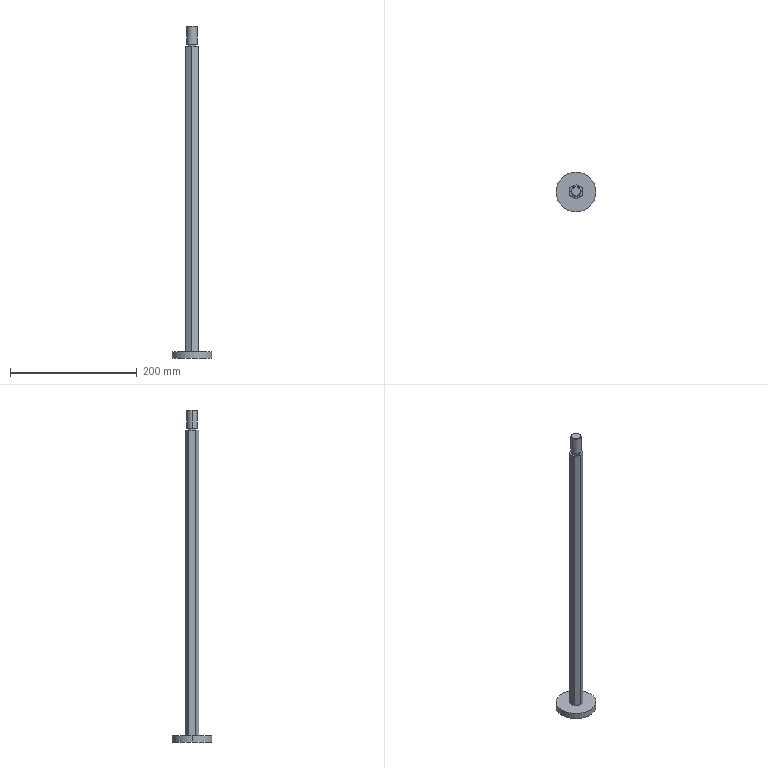Part | SolidWorks | features BaseBody 1 | 1 solid | 21 faces | box 63 x 63 x 524 mm | volume 188150 mm3 | plane 11 | cylinder 6 | cone 4 | commonest cylinder face diameters 14 x2 16 x2 63 x2
STEP:
#1=CARTESIAN_POINT('',(-242.,0.,321.531));
#2=VERTEX_POINT('',#1);
#3=CARTESIAN_POINT('',(-228.,0.,321.531));
#4=VERTEX_POINT('',#3);
#5=CARTESIAN_POINT('',(-235.,0.,321.531));
#6=DIRECTION('',(0.,0.,-1.));
#7=DIRECTION('',(-1.,0.,0.));
#8=AXIS2_PLACEMENT_3D('',#5,#6,#7);
#9=CIRCLE('',#8,7.);
#10=EDGE_CURVE('',#2,#4,#9,.T.);
#11=ORIENTED_EDGE('',*,*,#10,.T.);
#12=CARTESIAN_POINT('',(-228.,0.,319.281));
#13=VERTEX_POINT('',#12);
#14=CARTESIAN_POINT('',(-228.,0.,320.406));
#15=DIRECTION('',(0.,0.,-1.));
#16=VECTOR('',#15,1000.);
#17=LINE('',#14,#16);
#18=EDGE_CURVE('',#4,#13,#17,.T.);
#19=ORIENTED_EDGE('',*,*,#18,.T.);
#20=CARTESIAN_POINT('',(-242.,0.,319.281));
#21=VERTEX_POINT('',#20);
#22=CARTESIAN_POINT('',(-235.,0.,319.281));
#23=DIRECTION('',(0.,0.,-1.));
#24=DIRECTION('',(-1.,0.,0.));
#25=AXIS2_PLACEMENT_3D('',#22,#23,#24);
#26=CIRCLE('',#25,7.);
#27=EDGE_CURVE('',#21,#13,#26,.T.);
#28=ORIENTED_EDGE('',*,*,#27,.F.);
#29=CARTESIAN_POINT('',(-242.,0.,320.406));
#30=DIRECTION('',(0.,0.,-1.));
#31=VECTOR('',#30,1000.);
#32=LINE('',#29,#31);
#33=EDGE_CURVE('',#2,#21,#32,.T.);
#34=ORIENTED_EDGE('',*,*,#33,.F.);
#35=EDGE_LOOP('',(#11,#19,#28,#34));
#36=FACE_OUTER_BOUND('',#35,.T.);
#37=CARTESIAN_POINT('',(-235.,0.,320.406));
#38=DIRECTION('',(0.,0.,-1.));
#39=DIRECTION('',(-1.,0.,0.));
#40=AXIS2_PLACEMENT_3D('',#37,#38,#39);
#41=CYLINDRICAL_SURFACE('',#40,7.);
#42=ADVANCED_FACE('',(#36),#41,.T.);
#43=CARTESIAN_POINT('',(-203.5,0.,-162.719));
#44=VERTEX_POINT('',#43);
#45=CARTESIAN_POINT('',(-266.5,0.,-162.719));
#46=VERTEX_POINT('',#45);
#47=CARTESIAN_POINT('',(-235.,0.,-162.719));
#48=DIRECTION('',(0.,0.,1.));
#49=DIRECTION('',(-1.,0.,0.));
#50=AXIS2_PLACEMENT_3D('',#47,#48,#49);
#51=CIRCLE('',#50,31.5);
#52=EDGE_CURVE('',#44,#46,#51,.T.);
#53=ORIENTED_EDGE('',*,*,#52,.F.);
#54=CARTESIAN_POINT('',(-203.5,0.,-172.719));
#55=VERTEX_POINT('',#54);
#56=CARTESIAN_POINT('',(-203.5,0.,-167.719));
#57=DIRECTION('',(0.,0.,-1.));
#58=VECTOR('',#57,1000.);
#59=LINE('',#56,#58);
#60=EDGE_CURVE('',#44,#55,#59,.T.);
#61=ORIENTED_EDGE('',*,*,#60,.T.);
#62=CARTESIAN_POINT('',(-266.5,0.,-172.719));
#63=VERTEX_POINT('',#62);
#64=CARTESIAN_POINT('',(-235.,0.,-172.719));
#65=DIRECTION('',(0.,0.,1.));
#66=DIRECTION('',(-1.,0.,0.));
#67=AXIS2_PLACEMENT_3D('',#64,#65,#66);
#68=CIRCLE('',#67,31.5);
#69=EDGE_CURVE('',#55,#63,#68,.T.);
#70=ORIENTED_EDGE('',*,*,#69,.T.);
#71=CARTESIAN_POINT('',(-266.5,0.,-167.719));
#72=DIRECTION('',(0.,0.,-1.));
#73=VECTOR('',#72,1000.);
#74=LINE('',#71,#73);
#75=EDGE_CURVE('',#46,#63,#74,.T.);
#76=ORIENTED_EDGE('',*,*,#75,.F.);
#77=EDGE_LOOP('',(#53,#61,#70,#76));
#78=FACE_OUTER_BOUND('',#77,.T.);
#79=CARTESIAN_POINT('',(-235.,0.,-167.719));
#80=DIRECTION('',(0.,0.,-1.));
#81=DIRECTION('',(-1.,0.,0.));
#82=AXIS2_PLACEMENT_3D('',#79,#80,#81);
#83=CYLINDRICAL_SURFACE('',#82,31.5);
#84=ADVANCED_FACE('',(#78),#83,.T.);
#85=CARTESIAN_POINT('',(-242.08,0.,321.531));
#86=VERTEX_POINT('',#85);
#87=CARTESIAN_POINT('',(-227.92,0.,321.531));
#88=VERTEX_POINT('',#87);
#89=CARTESIAN_POINT('',(-235.,0.,321.531));
#90=DIRECTION('',(0.,0.,-1.));
#91=DIRECTION('',(1.,0.,0.));
#92=AXIS2_PLACEMENT_3D('',#89,#90,#91);
#93=CIRCLE('',#92,7.08);
#94=EDGE_CURVE('',#86,#88,#93,.T.);
#95=ORIENTED_EDGE('',*,*,#94,.F.);
#96=CARTESIAN_POINT('',(-243.,0.,322.451));
#97=VERTEX_POINT('',#96);
#98=CARTESIAN_POINT('',(-243.,0.,322.451));
#99=DIRECTION('',(-0.7071,0.,0.7071));
#100=VECTOR('',#99,1000.);
#101=LINE('',#98,#100);
#102=EDGE_CURVE('',#86,#97,#101,.T.);
#103=ORIENTED_EDGE('',*,*,#102,.T.);
#104=CARTESIAN_POINT('',(-227.,0.,322.451));
#105=VERTEX_POINT('',#104);
#106=CARTESIAN_POINT('',(-235.,0.,322.451));
#107=DIRECTION('',(0.,0.,-1.));
#108=DIRECTION('',(-0.866,-0.5,0.));
#109=AXIS2_PLACEMENT_3D('',#106,#107,#108);
#110=CIRCLE('',#109,8.);
#111=EDGE_CURVE('',#97,#105,#110,.T.);
#112=ORIENTED_EDGE('',*,*,#111,.T.);
#113=CARTESIAN_POINT('',(-227.,0.,322.451));
#114=DIRECTION('',(0.7071,0.,0.7071));
#115=VECTOR('',#114,1000.);
#116=LINE('',#113,#115);
#117=EDGE_CURVE('',#88,#105,#116,.T.);
#118=ORIENTED_EDGE('',*,*,#117,.F.);
#119=EDGE_LOOP('',(#95,#103,#112,#118));
#120=FACE_OUTER_BOUND('',#119,.T.);
#121=CARTESIAN_POINT('',(-235.,0.,322.451));
#122=DIRECTION('',(0.,0.,1.));
#123=DIRECTION('',(1.,0.,0.));
#124=AXIS2_PLACEMENT_3D('',#121,#122,#123);
#125=CONICAL_SURFACE('',#124,8.,0.7854);
#126=ADVANCED_FACE('',(#120),#125,.T.);
#127=CARTESIAN_POINT('',(-235.,8.,350.361));
#128=VERTEX_POINT('',#127);
#129=CARTESIAN_POINT('',(-227.,0.,350.361));
#130=VERTEX_POINT('',#129);
#131=CARTESIAN_POINT('',(-235.,0.,350.361));
#132=DIRECTION('',(0.,0.,-1.));
#133=DIRECTION('',(-1.,0.,0.));
#134=AXIS2_PLACEMENT_3D('',#131,#132,#133);
#135=CIRCLE('',#134,8.);
#136=EDGE_CURVE('',#128,#130,#135,.T.);
#137=ORIENTED_EDGE('',*,*,#136,.T.);
#138=CARTESIAN_POINT('',(-227.,0.,336.406));
#139=DIRECTION('',(0.,0.,-1.));
#140=VECTOR('',#139,1000.);
#141=LINE('',#138,#140);
#142=EDGE_CURVE('',#130,#105,#141,.T.);
#143=ORIENTED_EDGE('',*,*,#142,.T.);
#144=ORIENTED_EDGE('',*,*,#111,.F.);
#145=CARTESIAN_POINT('',(-243.,0.,350.361));
#146=VERTEX_POINT('',#145);
#147=CARTESIAN_POINT('',(-243.,0.,336.406));
#148=DIRECTION('',(0.,0.,-1.));
#149=VECTOR('',#148,1000.);
#150=LINE('',#147,#149);
#151=EDGE_CURVE('',#146,#97,#150,.T.);
#152=ORIENTED_EDGE('',*,*,#151,.F.);
#153=CARTESIAN_POINT('',(-235.,0.,350.361));
#154=DIRECTION('',(0.,0.,-1.));
#155=DIRECTION('',(-1.,0.,0.));
#156=AXIS2_PLACEMENT_3D('',#153,#154,#155);
#157=CIRCLE('',#156,8.);
#158=EDGE_CURVE('',#146,#128,#157,.T.);
#159=ORIENTED_EDGE('',*,*,#158,.T.);
#160=EDGE_LOOP('',(#137,#143,#144,#152,#159));
#161=FACE_OUTER_BOUND('',#160,.T.);
#162=CARTESIAN_POINT('',(-235.,0.,336.406));
#163=DIRECTION('',(0.,0.,-1.));
#164=DIRECTION('',(-1.,0.,0.));
#165=AXIS2_PLACEMENT_3D('',#162,#163,#164);
#166=CYLINDRICAL_SURFACE('',#165,8.);
#167=ADVANCED_FACE('',(#161),#166,.T.);
#168=CARTESIAN_POINT('',(-235.,7.08,351.281));
#169=VERTEX_POINT('',#168);
#170=CARTESIAN_POINT('',(-235.,-7.08,351.281));
#171=VERTEX_POINT('',#170);
#172=CARTESIAN_POINT('',(-235.,0.,351.281));
#173=DIRECTION('',(0.,0.,-1.));
#174=DIRECTION('',(0.,1.,0.));
#175=AXIS2_PLACEMENT_3D('',#172,#173,#174);
#176=CIRCLE('',#175,7.08);
#177=EDGE_CURVE('',#169,#171,#176,.T.);
#178=ORIENTED_EDGE('',*,*,#177,.T.);
#179=CARTESIAN_POINT('',(-235.,-8.,350.361));
#180=VERTEX_POINT('',#179);
#181=CARTESIAN_POINT('',(-235.,-8.,350.361));
#182=DIRECTION('',(0.,-0.7071,-0.7071));
#183=VECTOR('',#182,1000.);
#184=LINE('',#181,#183);
#185=EDGE_CURVE('',#171,#180,#184,.T.);
#186=ORIENTED_EDGE('',*,*,#185,.T.);
#187=CARTESIAN_POINT('',(-235.,0.,350.361));
#188=DIRECTION('',(0.,0.,-1.));
#189=DIRECTION('',(-1.,0.,0.));
#190=AXIS2_PLACEMENT_3D('',#187,#188,#189);
#191=CIRCLE('',#190,8.);
#192=EDGE_CURVE('',#130,#180,#191,.T.);
#193=ORIENTED_EDGE('',*,*,#192,.F.);
#194=ORIENTED_EDGE('',*,*,#136,.F.);
#195=CARTESIAN_POINT('',(-235.,8.,350.361));
#196=DIRECTION('',(0.,0.7071,-0.7071));
#197=VECTOR('',#196,1000.);
#198=LINE('',#195,#197);
#199=EDGE_CURVE('',#169,#128,#198,.T.);
#200=ORIENTED_EDGE('',*,*,#199,.F.);
#201=EDGE_LOOP('',(#178,#186,#193,#194,#200));
#202=FACE_OUTER_BOUND('',#201,.T.);
#203=CARTESIAN_POINT('',(-235.,0.,350.361));
#204=DIRECTION('',(0.,0.,-1.));
#205=DIRECTION('',(0.,1.,0.));
#206=AXIS2_PLACEMENT_3D('',#203,#204,#205);
#207=CONICAL_SURFACE('',#206,8.,0.7854);
#208=ADVANCED_FACE('',(#202),#207,.T.);
#209=CARTESIAN_POINT('',(-235.,-10.97,319.281));
#210=VERTEX_POINT('',#209);
#211=CARTESIAN_POINT('',(-225.5,-5.485,319.281));
#212=VERTEX_POINT('',#211);
#213=CARTESIAN_POINT('',(-225.5,-5.485,319.281));
#214=DIRECTION('',(0.866,0.5,0.));
#215=VECTOR('',#214,1000.);
#216=LINE('',#213,#215);
#217=EDGE_CURVE('',#210,#212,#216,.T.);
#218=ORIENTED_EDGE('',*,*,#217,.F.);
#219=CARTESIAN_POINT('',(-235.,-10.97,-162.719));
#220=VERTEX_POINT('',#219);
#221=CARTESIAN_POINT('',(-235.,-10.97,319.281));
#222=DIRECTION('',(0.,0.,1.));
#223=VECTOR('',#222,1000.);
#224=LINE('',#221,#223);
#225=EDGE_CURVE('',#220,#210,#224,.T.);
#226=ORIENTED_EDGE('',*,*,#225,.F.);
#227=CARTESIAN_POINT('',(-225.5,-5.485,-162.719));
#228=VERTEX_POINT('',#227);
#229=CARTESIAN_POINT('',(-225.5,-5.485,-162.719));
#230=DIRECTION('',(-0.866,-0.5,0.));
#231=VECTOR('',#230,1000.);
#232=LINE('',#229,#231);
#233=EDGE_CURVE('',#228,#220,#232,.T.);
#234=ORIENTED_EDGE('',*,*,#233,.F.);
#235=CARTESIAN_POINT('',(-225.5,-5.485,319.281));
#236=DIRECTION('',(0.,0.,-1.));
#237=VECTOR('',#236,1000.);
#238=LINE('',#235,#237);
#239=EDGE_CURVE('',#212,#228,#238,.T.);
#240=ORIENTED_EDGE('',*,*,#239,.F.);
#241=EDGE_LOOP('',(#218,#226,#234,#240));
#242=FACE_OUTER_BOUND('',#241,.T.);
#243=CARTESIAN_POINT('',(-225.5,-5.485,319.281));
#244=DIRECTION('',(-0.5,0.866,0.));
#245=DIRECTION('',(-0.866,-0.5,0.));
#246=AXIS2_PLACEMENT_3D('',#243,#244,#245);
#247=PLANE('',#246);
#248=ADVANCED_FACE('',(#242),#247,.F.);
#249=CARTESIAN_POINT('',(-225.5,5.485,319.281));
#250=VERTEX_POINT('',#249);
#251=CARTESIAN_POINT('',(-225.5,5.485,319.281));
#252=DIRECTION('',(0.,1.,0.));
#253=VECTOR('',#252,1000.);
#254=LINE('',#251,#253);
#255=EDGE_CURVE('',#212,#250,#254,.T.);
#256=ORIENTED_EDGE('',*,*,#255,.F.);
#257=ORIENTED_EDGE('',*,*,#239,.T.);
#258=CARTESIAN_POINT('',(-225.5,5.485,-162.719));
#259=VERTEX_POINT('',#258);
#260=CARTESIAN_POINT('',(-225.5,5.485,-162.719));
#261=DIRECTION('',(0.,-1.,0.));
#262=VECTOR('',#261,1000.);
#263=LINE('',#260,#262);
#264=EDGE_CURVE('',#259,#228,#263,.T.);
#265=ORIENTED_EDGE('',*,*,#264,.F.);
#266=CARTESIAN_POINT('',(-225.5,5.485,319.281));
#267=DIRECTION('',(0.,0.,-1.));
#268=VECTOR('',#267,1000.);
#269=LINE('',#266,#268);
#270=EDGE_CURVE('',#250,#259,#269,.T.);
#271=ORIENTED_EDGE('',*,*,#270,.F.);
#272=EDGE_LOOP('',(#256,#257,#265,#271));
#273=FACE_OUTER_BOUND('',#272,.T.);
#274=CARTESIAN_POINT('',(-225.5,5.485,319.281));
#275=DIRECTION('',(-1.,0.,0.));
#276=DIRECTION('',(0.,0.,1.));
#277=AXIS2_PLACEMENT_3D('',#274,#275,#276);
#278=PLANE('',#277);
#279=ADVANCED_FACE('',(#273),#278,.F.);
#280=CARTESIAN_POINT('',(-235.,10.97,319.281));
#281=VERTEX_POINT('',#280);
#282=CARTESIAN_POINT('',(-244.5,5.485,319.281));
#283=VERTEX_POINT('',#282);
#284=CARTESIAN_POINT('',(-235.,10.97,319.281));
#285=DIRECTION('',(-0.866,-0.5,0.));
#286=VECTOR('',#285,1000.);
#287=LINE('',#284,#286);
#288=EDGE_CURVE('',#281,#283,#287,.T.);
#289=ORIENTED_EDGE('',*,*,#288,.T.);
#290=CARTESIAN_POINT('',(-244.5,-5.485,319.281));
#291=VERTEX_POINT('',#290);
#292=CARTESIAN_POINT('',(-244.5,9.613,319.281));
#293=DIRECTION('',(0.,-1.,0.));
#294=VECTOR('',#293,1000.);
#295=LINE('',#292,#294);
#296=EDGE_CURVE('',#283,#291,#295,.T.);
#297=ORIENTED_EDGE('',*,*,#296,.T.);
#298=CARTESIAN_POINT('',(-244.5,-5.485,319.281));
#299=DIRECTION('',(0.866,-0.5,0.));
#300=VECTOR('',#299,1000.);
#301=LINE('',#298,#300);
#302=EDGE_CURVE('',#291,#210,#301,.T.);
#303=ORIENTED_EDGE('',*,*,#302,.T.);
#304=ORIENTED_EDGE('',*,*,#217,.T.);
#305=ORIENTED_EDGE('',*,*,#255,.T.);
#306=CARTESIAN_POINT('',(-225.5,5.485,319.281));
#307=DIRECTION('',(-0.866,0.5,0.));
#308=VECTOR('',#307,1000.);
#309=LINE('',#306,#308);
#310=EDGE_CURVE('',#250,#281,#309,.T.);
#311=ORIENTED_EDGE('',*,*,#310,.T.);
#312=EDGE_LOOP('',(#289,#297,#303,#304,#305,#311));
#313=FACE_OUTER_BOUND('',#312,.T.);
#314=ORIENTED_EDGE('',*,*,#27,.T.);
#315=CARTESIAN_POINT('',(-235.,0.,319.281));
#316=DIRECTION('',(0.,0.,-1.));
#317=DIRECTION('',(-1.,0.,0.));
#318=AXIS2_PLACEMENT_3D('',#315,#316,#317);
#319=CIRCLE('',#318,7.);
#320=EDGE_CURVE('',#13,#21,#319,.T.);
#321=ORIENTED_EDGE('',*,*,#320,.T.);
#322=EDGE_LOOP('',(#314,#321));
#323=FACE_BOUND('',#322,.T.);
#324=CARTESIAN_POINT('',(-240.55,9.613,319.281));
#325=DIRECTION('',(0.,0.,1.));
#326=DIRECTION('',(1.,0.,0.));
#327=AXIS2_PLACEMENT_3D('',#324,#325,#326);
#328=PLANE('',#327);
#329=ADVANCED_FACE('',(#313,#323),#328,.T.);
#330=ORIENTED_EDGE('',*,*,#302,.F.);
#331=CARTESIAN_POINT('',(-244.5,-5.485,-162.719));
#332=VERTEX_POINT('',#331);
#333=CARTESIAN_POINT('',(-244.5,-5.485,319.281));
#334=DIRECTION('',(0.,0.,1.));
#335=VECTOR('',#334,1000.);
#336=LINE('',#333,#335);
#337=EDGE_CURVE('',#332,#291,#336,.T.);
#338=ORIENTED_EDGE('',*,*,#337,.F.);
#339=CARTESIAN_POINT('',(-235.,-10.97,-162.719));
#340=DIRECTION('',(-0.866,0.5,0.));
#341=VECTOR('',#340,1000.);
#342=LINE('',#339,#341);
#343=EDGE_CURVE('',#220,#332,#342,.T.);
#344=ORIENTED_EDGE('',*,*,#343,.F.);
#345=ORIENTED_EDGE('',*,*,#225,.T.);
#346=EDGE_LOOP('',(#330,#338,#344,#345));
#347=FACE_OUTER_BOUND('',#346,.T.);
#348=CARTESIAN_POINT('',(-235.,-10.97,319.281));
#349=DIRECTION('',(0.5,0.866,0.));
#350=DIRECTION('',(-0.866,0.5,0.));
#351=AXIS2_PLACEMENT_3D('',#348,#349,#350);
#352=PLANE('',#351);
#353=ADVANCED_FACE('',(#347),#352,.F.);
#354=ORIENTED_EDGE('',*,*,#343,.T.);
#355=CARTESIAN_POINT('',(-244.5,5.485,-162.719));
#356=VERTEX_POINT('',#355);
#357=CARTESIAN_POINT('',(-244.5,20.222,-162.719));
#358=DIRECTION('',(0.,1.,0.));
#359=VECTOR('',#358,1000.);
#360=LINE('',#357,#359);
#361=EDGE_CURVE('',#332,#356,#360,.T.);
#362=ORIENTED_EDGE('',*,*,#361,.T.);
#363=CARTESIAN_POINT('',(-235.,10.97,-162.719));
#364=VERTEX_POINT('',#363);
#365=CARTESIAN_POINT('',(-244.5,5.485,-162.719));
#366=DIRECTION('',(0.866,0.5,0.));
#367=VECTOR('',#366,1000.);
#368=LINE('',#365,#367);
#369=EDGE_CURVE('',#356,#364,#368,.T.);
#370=ORIENTED_EDGE('',*,*,#369,.T.);
#371=CARTESIAN_POINT('',(-235.,10.97,-162.719));
#372=DIRECTION('',(0.866,-0.5,0.));
#373=VECTOR('',#372,1000.);
#374=LINE('',#371,#373);
#375=EDGE_CURVE('',#364,#259,#374,.T.);
#376=ORIENTED_EDGE('',*,*,#375,.T.);
#377=ORIENTED_EDGE('',*,*,#264,.T.);
#378=ORIENTED_EDGE('',*,*,#233,.T.);
#379=EDGE_LOOP('',(#354,#362,#370,#376,#377,#378));
#380=FACE_BOUND('',#379,.T.);
#381=CARTESIAN_POINT('',(-235.,0.,-162.719));
#382=DIRECTION('',(0.,0.,1.));
#383=DIRECTION('',(-1.,0.,0.));
#384=AXIS2_PLACEMENT_3D('',#381,#382,#383);
#385=CIRCLE('',#384,31.5);
#386=EDGE_CURVE('',#46,#44,#385,.T.);
#387=ORIENTED_EDGE('',*,*,#386,.T.);
#388=ORIENTED_EDGE('',*,*,#52,.T.);
#389=EDGE_LOOP('',(#387,#388));
#390=FACE_OUTER_BOUND('',#389,.T.);
#391=CARTESIAN_POINT('',(-246.675,20.222,-162.719));
#392=DIRECTION('',(0.,0.,1.));
#393=DIRECTION('',(1.,0.,0.));
#394=AXIS2_PLACEMENT_3D('',#391,#392,#393);
#395=PLANE('',#394);
#396=ADVANCED_FACE('',(#380,#390),#395,.T.);
#397=ORIENTED_EDGE('',*,*,#310,.F.);
#398=ORIENTED_EDGE('',*,*,#270,.T.);
#399=ORIENTED_EDGE('',*,*,#375,.F.);
#400=CARTESIAN_POINT('',(-235.,10.97,319.281));
#401=DIRECTION('',(0.,0.,-1.));
#402=VECTOR('',#401,1000.);
#403=LINE('',#400,#402);
#404=EDGE_CURVE('',#281,#364,#403,.T.);
#405=ORIENTED_EDGE('',*,*,#404,.F.);
#406=EDGE_LOOP('',(#397,#398,#399,#405));
#407=FACE_OUTER_BOUND('',#406,.T.);
#408=CARTESIAN_POINT('',(-235.,10.97,319.281));
#409=DIRECTION('',(-0.5,-0.866,0.));
#410=DIRECTION('',(0.866,-0.5,0.));
#411=AXIS2_PLACEMENT_3D('',#408,#409,#410);
#412=PLANE('',#411);
#413=ADVANCED_FACE('',(#407),#412,.F.);
#414=ORIENTED_EDGE('',*,*,#296,.F.);
#415=CARTESIAN_POINT('',(-244.5,5.485,319.281));
#416=DIRECTION('',(0.,0.,1.));
#417=VECTOR('',#416,1000.);
#418=LINE('',#415,#417);
#419=EDGE_CURVE('',#356,#283,#418,.T.);
#420=ORIENTED_EDGE('',*,*,#419,.F.);
#421=ORIENTED_EDGE('',*,*,#361,.F.);
#422=ORIENTED_EDGE('',*,*,#337,.T.);
#423=EDGE_LOOP('',(#414,#420,#421,#422));
#424=FACE_OUTER_BOUND('',#423,.T.);
#425=CARTESIAN_POINT('',(-244.5,-5.485,319.281));
#426=DIRECTION('',(1.,0.,0.));
#427=DIRECTION('',(0.,0.,-1.));
#428=AXIS2_PLACEMENT_3D('',#425,#426,#427);
#429=PLANE('',#428);
#430=ADVANCED_FACE('',(#424),#429,.F.);
#431=ORIENTED_EDGE('',*,*,#288,.F.);
#432=ORIENTED_EDGE('',*,*,#404,.T.);
#433=ORIENTED_EDGE('',*,*,#369,.F.);
#434=ORIENTED_EDGE('',*,*,#419,.T.);
#435=EDGE_LOOP('',(#431,#432,#433,#434));
#436=FACE_OUTER_BOUND('',#435,.T.);
#437=CARTESIAN_POINT('',(-244.5,5.485,319.281));
#438=DIRECTION('',(0.5,-0.866,0.));
#439=DIRECTION('',(0.866,0.5,0.));
#440=AXIS2_PLACEMENT_3D('',#437,#438,#439);
#441=PLANE('',#440);
#442=ADVANCED_FACE('',(#436),#441,.F.);
#443=ORIENTED_EDGE('',*,*,#18,.F.);
#444=CARTESIAN_POINT('',(-235.,0.,321.531));
#445=DIRECTION('',(0.,0.,-1.));
#446=DIRECTION('',(-1.,0.,0.));
#447=AXIS2_PLACEMENT_3D('',#444,#445,#446);
#448=CIRCLE('',#447,7.);
#449=EDGE_CURVE('',#4,#2,#448,.T.);
#450=ORIENTED_EDGE('',*,*,#449,.T.);
#451=ORIENTED_EDGE('',*,*,#33,.T.);
#452=ORIENTED_EDGE('',*,*,#320,.F.);
#453=EDGE_LOOP('',(#443,#450,#451,#452));
#454=FACE_OUTER_BOUND('',#453,.T.);
#455=CARTESIAN_POINT('',(-235.,0.,320.406));
#456=DIRECTION('',(0.,0.,-1.));
#457=DIRECTION('',(-1.,0.,0.));
#458=AXIS2_PLACEMENT_3D('',#455,#456,#457);
#459=CYLINDRICAL_SURFACE('',#458,7.);
#460=ADVANCED_FACE('',(#454),#459,.T.);
#461=ORIENTED_EDGE('',*,*,#60,.F.);
#462=ORIENTED_EDGE('',*,*,#386,.F.);
#463=ORIENTED_EDGE('',*,*,#75,.T.);
#464=CARTESIAN_POINT('',(-235.,0.,-172.719));
#465=DIRECTION('',(0.,0.,1.));
#466=DIRECTION('',(-1.,0.,0.));
#467=AXIS2_PLACEMENT_3D('',#464,#465,#466);
#468=CIRCLE('',#467,31.5);
#469=EDGE_CURVE('',#63,#55,#468,.T.);
#470=ORIENTED_EDGE('',*,*,#469,.T.);
#471=EDGE_LOOP('',(#461,#462,#463,#470));
#472=FACE_OUTER_BOUND('',#471,.T.);
#473=CARTESIAN_POINT('',(-235.,0.,-167.719));
#474=DIRECTION('',(0.,0.,-1.));
#475=DIRECTION('',(-1.,0.,0.));
#476=AXIS2_PLACEMENT_3D('',#473,#474,#475);
#477=CYLINDRICAL_SURFACE('',#476,31.5);
#478=ADVANCED_FACE('',(#472),#477,.T.);
#479=CARTESIAN_POINT('',(-235.,0.,321.531));
#480=DIRECTION('',(0.,0.,-1.));
#481=DIRECTION('',(1.,0.,0.));
#482=AXIS2_PLACEMENT_3D('',#479,#480,#481);
#483=CIRCLE('',#482,7.08);
#484=EDGE_CURVE('',#88,#86,#483,.T.);
#485=ORIENTED_EDGE('',*,*,#484,.T.);
#486=ORIENTED_EDGE('',*,*,#94,.T.);
#487=EDGE_LOOP('',(#485,#486));
#488=FACE_OUTER_BOUND('',#487,.T.);
#489=ORIENTED_EDGE('',*,*,#10,.F.);
#490=ORIENTED_EDGE('',*,*,#449,.F.);
#491=EDGE_LOOP('',(#489,#490));
#492=FACE_BOUND('',#491,.T.);
#493=CARTESIAN_POINT('',(-238.52,6.097,321.531));
#494=DIRECTION('',(0.,0.,-1.));
#495=DIRECTION('',(-1.,0.,0.));
#496=AXIS2_PLACEMENT_3D('',#493,#494,#495);
#497=PLANE('',#496);
#498=ADVANCED_FACE('',(#488,#492),#497,.T.);
#499=ORIENTED_EDGE('',*,*,#469,.F.);
#500=ORIENTED_EDGE('',*,*,#69,.F.);
#501=EDGE_LOOP('',(#499,#500));
#502=FACE_OUTER_BOUND('',#501,.T.);
#503=CARTESIAN_POINT('',(-242.875,13.64,-172.719));
#504=DIRECTION('',(0.,0.,-1.));
#505=DIRECTION('',(-1.,0.,0.));
#506=AXIS2_PLACEMENT_3D('',#503,#504,#505);
#507=PLANE('',#506);
#508=ADVANCED_FACE('',(#502),#507,.T.);
#509=ORIENTED_EDGE('',*,*,#102,.F.);
#510=ORIENTED_EDGE('',*,*,#484,.F.);
#511=ORIENTED_EDGE('',*,*,#117,.T.);
#512=CARTESIAN_POINT('',(-235.,0.,322.451));
#513=DIRECTION('',(0.,0.,-1.));
#514=DIRECTION('',(-0.866,-0.5,0.));
#515=AXIS2_PLACEMENT_3D('',#512,#513,#514);
#516=CIRCLE('',#515,8.);
#517=EDGE_CURVE('',#105,#97,#516,.T.);
#518=ORIENTED_EDGE('',*,*,#517,.T.);
#519=EDGE_LOOP('',(#509,#510,#511,#518));
#520=FACE_OUTER_BOUND('',#519,.T.);
#521=CARTESIAN_POINT('',(-235.,0.,322.451));
#522=DIRECTION('',(0.,0.,1.));
#523=DIRECTION('',(1.,0.,0.));
#524=AXIS2_PLACEMENT_3D('',#521,#522,#523);
#525=CONICAL_SURFACE('',#524,8.,0.7854);
#526=ADVANCED_FACE('',(#520),#525,.T.);
#527=ORIENTED_EDGE('',*,*,#142,.F.);
#528=ORIENTED_EDGE('',*,*,#192,.T.);
#529=CARTESIAN_POINT('',(-235.,0.,350.361));
#530=DIRECTION('',(0.,0.,-1.));
#531=DIRECTION('',(-1.,0.,0.));
#532=AXIS2_PLACEMENT_3D('',#529,#530,#531);
#533=CIRCLE('',#532,8.);
#534=EDGE_CURVE('',#180,#146,#533,.T.);
#535=ORIENTED_EDGE('',*,*,#534,.T.);
#536=ORIENTED_EDGE('',*,*,#151,.T.);
#537=ORIENTED_EDGE('',*,*,#517,.F.);
#538=EDGE_LOOP('',(#527,#528,#535,#536,#537));
#539=FACE_OUTER_BOUND('',#538,.T.);
#540=CARTESIAN_POINT('',(-235.,0.,336.406));
#541=DIRECTION('',(0.,0.,-1.));
#542=DIRECTION('',(-1.,0.,0.));
#543=AXIS2_PLACEMENT_3D('',#540,#541,#542);
#544=CYLINDRICAL_SURFACE('',#543,8.);
#545=ADVANCED_FACE('',(#539),#544,.T.);
#546=ORIENTED_EDGE('',*,*,#185,.F.);
#547=CARTESIAN_POINT('',(-235.,0.,351.281));
#548=DIRECTION('',(0.,0.,-1.));
#549=DIRECTION('',(0.,1.,0.));
#550=AXIS2_PLACEMENT_3D('',#547,#548,#549);
#551=CIRCLE('',#550,7.08);
#552=EDGE_CURVE('',#171,#169,#551,.T.);
#553=ORIENTED_EDGE('',*,*,#552,.T.);
#554=ORIENTED_EDGE('',*,*,#199,.T.);
#555=ORIENTED_EDGE('',*,*,#158,.F.);
#556=ORIENTED_EDGE('',*,*,#534,.F.);
#557=EDGE_LOOP('',(#546,#553,#554,#555,#556));
#558=FACE_OUTER_BOUND('',#557,.T.);
#559=CARTESIAN_POINT('',(-235.,0.,350.361));
#560=DIRECTION('',(0.,0.,-1.));
#561=DIRECTION('',(0.,1.,0.));
#562=AXIS2_PLACEMENT_3D('',#559,#560,#561);
#563=CONICAL_SURFACE('',#562,8.,0.7854);
#564=ADVANCED_FACE('',(#558),#563,.T.);
#565=ORIENTED_EDGE('',*,*,#177,.F.);
#566=ORIENTED_EDGE('',*,*,#552,.F.);
#567=EDGE_LOOP('',(#565,#566));
#568=FACE_OUTER_BOUND('',#567,.T.);
#569=CARTESIAN_POINT('',(-236.77,3.066,351.281));
#570=DIRECTION('',(0.,0.,1.));
#571=DIRECTION('',(1.,0.,0.));
#572=AXIS2_PLACEMENT_3D('',#569,#570,#571);
#573=PLANE('',#572);
#574=ADVANCED_FACE('',(#568),#573,.T.);
#575=CLOSED_SHELL('',(#42,#84,#126,#167,#208,#248,#279,#329,#353,#396,#413,#430,#442,#460,#478,#498,#508,#526,#545,#564,#574));
#576=MANIFOLD_SOLID_BREP('',#575);
#577=CARTESIAN_POINT('',(0.,0.,0.));
#578=DIRECTION('',(0.,0.,1.));
#579=DIRECTION('',(1.,0.,0.));
#580=AXIS2_PLACEMENT_3D('',#577,#578,#579);
#581=(LENGTH_UNIT()NAMED_UNIT(*)SI_UNIT(.MILLI.,.METRE.));
#582=UNCERTAINTY_MEASURE_WITH_UNIT(LENGTH_MEASURE(0.00001),#581,'','');
#583=(NAMED_UNIT(*)PLANE_ANGLE_UNIT()SI_UNIT($,.RADIAN.));
#584=(NAMED_UNIT(*)SI_UNIT($,.STERADIAN.)SOLID_ANGLE_UNIT());
#585=(GEOMETRIC_REPRESENTATION_CONTEXT(3)GLOBAL_UNCERTAINTY_ASSIGNED_CONTEXT((#582))GLOBAL_UNIT_ASSIGNED_CONTEXT((#581,#583,#584))REPRESENTATION_CONTEXT('',''));
#586=ADVANCED_BREP_SHAPE_REPRESENTATION('',(#576,#580),#585);